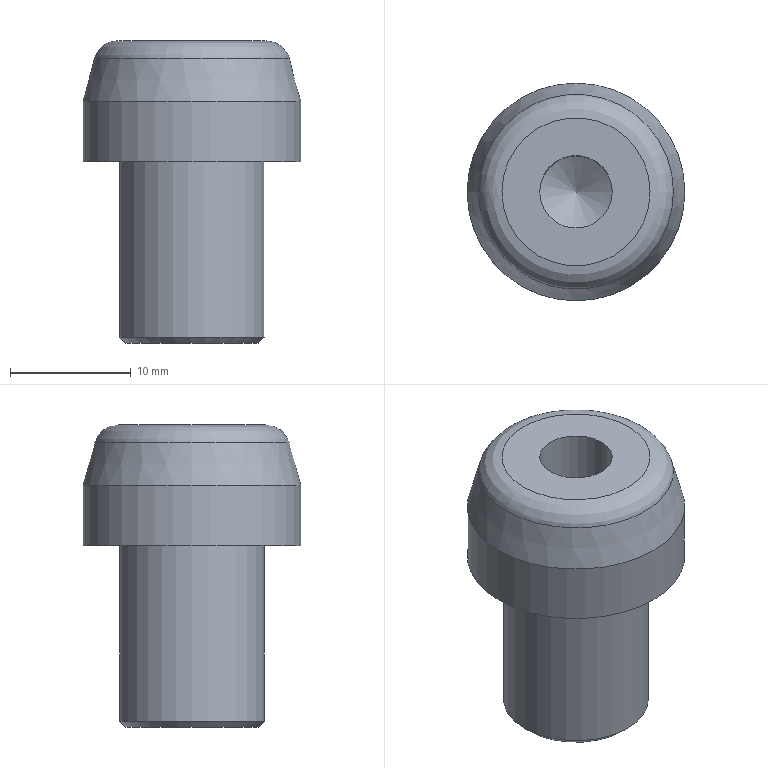Part | NX | features solid 2 | 1 solid | 10 faces | box 18 x 18 x 25 mm | volume 3736 mm3 | plane 3 | cylinder 3 | cone 3 | torus 1 | commonest cylinder face diameters 6 x1 12 x1 18 x1
STEP:
#1=CARTESIAN_POINT('',(83.131,-155.39,65.396));
#2=VERTEX_POINT('',#1);
#3=CARTESIAN_POINT('',(89.131,-155.39,65.396));
#4=DIRECTION('',(0.,0.,-1.));
#5=DIRECTION('',(-1.,0.,0.));
#6=AXIS2_PLACEMENT_3D('',#3,#4,#5);
#7=CIRCLE('',#6,6.);
#8=EDGE_CURVE('',#2,#2,#7,.T.);
#9=ORIENTED_EDGE('',*,*,#8,.F.);
#10=EDGE_LOOP('',(#9));
#11=FACE_BOUND('',#10,.T.);
#12=CARTESIAN_POINT('',(98.131,-155.39,65.396));
#13=VERTEX_POINT('',#12);
#14=CARTESIAN_POINT('',(89.131,-155.39,65.396));
#15=DIRECTION('',(0.,0.,1.));
#16=DIRECTION('',(1.,0.,0.));
#17=AXIS2_PLACEMENT_3D('',#14,#15,#16);
#18=CIRCLE('',#17,9.);
#19=EDGE_CURVE('',#13,#13,#18,.T.);
#20=ORIENTED_EDGE('',*,*,#19,.F.);
#21=EDGE_LOOP('',(#20));
#22=FACE_BOUND('',#21,.T.);
#23=CARTESIAN_POINT('',(89.131,-155.39,65.396));
#24=DIRECTION('',(0.,0.,-1.));
#25=DIRECTION('',(-1.,0.,0.));
#26=AXIS2_PLACEMENT_3D('',#23,#24,#25);
#27=PLANE('',#26);
#28=ADVANCED_FACE('',(#11,#22),#27,.T.);
#29=CARTESIAN_POINT('',(80.131,-155.39,70.396));
#30=VERTEX_POINT('',#29);
#31=CARTESIAN_POINT('',(89.131,-155.39,70.396));
#32=DIRECTION('',(0.,0.,-1.));
#33=DIRECTION('',(-1.,0.,0.));
#34=AXIS2_PLACEMENT_3D('',#31,#32,#33);
#35=CIRCLE('',#34,9.);
#36=EDGE_CURVE('',#30,#30,#35,.T.);
#37=ORIENTED_EDGE('',*,*,#36,.T.);
#38=EDGE_LOOP('',(#37));
#39=FACE_BOUND('',#38,.T.);
#40=ORIENTED_EDGE('',*,*,#19,.T.);
#41=EDGE_LOOP('',(#40));
#42=FACE_BOUND('',#41,.T.);
#43=CARTESIAN_POINT('',(89.131,-155.39,65.396));
#44=DIRECTION('',(0.,0.,1.));
#45=DIRECTION('',(1.,0.,0.));
#46=AXIS2_PLACEMENT_3D('',#43,#44,#45);
#47=CYLINDRICAL_SURFACE('',#46,9.);
#48=ADVANCED_FACE('',(#39,#42),#47,.T.);
#49=CARTESIAN_POINT('',(81.073,-155.39,73.914));
#50=VERTEX_POINT('',#49);
#51=CARTESIAN_POINT('',(89.131,-155.39,73.914));
#52=DIRECTION('',(0.,0.,-1.));
#53=DIRECTION('',(-1.,0.,0.));
#54=AXIS2_PLACEMENT_3D('',#51,#52,#53);
#55=CIRCLE('',#54,8.057);
#56=EDGE_CURVE('',#50,#50,#55,.T.);
#57=ORIENTED_EDGE('',*,*,#56,.T.);
#58=EDGE_LOOP('',(#57));
#59=FACE_BOUND('',#58,.T.);
#60=ORIENTED_EDGE('',*,*,#36,.F.);
#61=EDGE_LOOP('',(#60));
#62=FACE_BOUND('',#61,.T.);
#63=CARTESIAN_POINT('',(89.131,-155.39,70.396));
#64=DIRECTION('',(0.,0.,-1.));
#65=DIRECTION('',(1.,0.,0.));
#66=AXIS2_PLACEMENT_3D('',#63,#64,#65);
#67=CONICAL_SURFACE('',#66,9.,0.2618);
#68=ADVANCED_FACE('',(#59,#62),#67,.T.);
#69=CARTESIAN_POINT('',(86.131,-155.39,75.396));
#70=VERTEX_POINT('',#69);
#71=CARTESIAN_POINT('',(89.131,-155.39,75.396));
#72=DIRECTION('',(0.,0.,-1.));
#73=DIRECTION('',(-1.,0.,0.));
#74=AXIS2_PLACEMENT_3D('',#71,#72,#73);
#75=CIRCLE('',#74,3.);
#76=EDGE_CURVE('',#70,#70,#75,.T.);
#77=ORIENTED_EDGE('',*,*,#76,.T.);
#78=EDGE_LOOP('',(#77));
#79=FACE_BOUND('',#78,.T.);
#80=CARTESIAN_POINT('',(83.005,-155.39,75.396));
#81=VERTEX_POINT('',#80);
#82=CARTESIAN_POINT('',(89.131,-155.39,75.396));
#83=DIRECTION('',(0.,0.,-1.));
#84=DIRECTION('',(-1.,0.,0.));
#85=AXIS2_PLACEMENT_3D('',#82,#83,#84);
#86=CIRCLE('',#85,6.126);
#87=EDGE_CURVE('',#81,#81,#86,.F.);
#88=ORIENTED_EDGE('',*,*,#87,.T.);
#89=EDGE_LOOP('',(#88));
#90=FACE_BOUND('',#89,.T.);
#91=CARTESIAN_POINT('',(89.131,-155.39,75.396));
#92=DIRECTION('',(0.,0.,-1.));
#93=DIRECTION('',(-1.,0.,0.));
#94=AXIS2_PLACEMENT_3D('',#91,#92,#93);
#95=PLANE('',#94);
#96=ADVANCED_FACE('',(#79,#90),#95,.F.);
#97=CARTESIAN_POINT('',(83.631,-155.39,50.396));
#98=VERTEX_POINT('',#97);
#99=CARTESIAN_POINT('',(89.131,-155.39,50.396));
#100=DIRECTION('',(0.,0.,-1.));
#101=DIRECTION('',(-1.,0.,0.));
#102=AXIS2_PLACEMENT_3D('',#99,#100,#101);
#103=CIRCLE('',#102,5.5);
#104=EDGE_CURVE('',#98,#98,#103,.T.);
#105=ORIENTED_EDGE('',*,*,#104,.T.);
#106=EDGE_LOOP('',(#105));
#107=FACE_BOUND('',#106,.T.);
#108=CARTESIAN_POINT('',(89.131,-155.39,50.396));
#109=DIRECTION('',(0.,0.,-1.));
#110=DIRECTION('',(-1.,0.,0.));
#111=AXIS2_PLACEMENT_3D('',#108,#109,#110);
#112=PLANE('',#111);
#113=ADVANCED_FACE('',(#107),#112,.T.);
#114=CARTESIAN_POINT('',(83.131,-155.39,50.896));
#115=VERTEX_POINT('',#114);
#116=CARTESIAN_POINT('',(89.131,-155.39,50.896));
#117=DIRECTION('',(0.,0.,-1.));
#118=DIRECTION('',(-1.,0.,0.));
#119=AXIS2_PLACEMENT_3D('',#116,#117,#118);
#120=CIRCLE('',#119,6.);
#121=EDGE_CURVE('',#115,#115,#120,.F.);
#122=ORIENTED_EDGE('',*,*,#121,.T.);
#123=EDGE_LOOP('',(#122));
#124=FACE_BOUND('',#123,.T.);
#125=ORIENTED_EDGE('',*,*,#8,.T.);
#126=EDGE_LOOP('',(#125));
#127=FACE_BOUND('',#126,.T.);
#128=CARTESIAN_POINT('',(89.131,-155.39,65.396));
#129=DIRECTION('',(0.,0.,-1.));
#130=DIRECTION('',(-1.,0.,0.));
#131=AXIS2_PLACEMENT_3D('',#128,#129,#130);
#132=CYLINDRICAL_SURFACE('',#131,6.);
#133=ADVANCED_FACE('',(#124,#127),#132,.T.);
#134=ORIENTED_EDGE('',*,*,#121,.F.);
#135=EDGE_LOOP('',(#134));
#136=FACE_BOUND('',#135,.T.);
#137=ORIENTED_EDGE('',*,*,#104,.F.);
#138=EDGE_LOOP('',(#137));
#139=FACE_BOUND('',#138,.T.);
#140=CARTESIAN_POINT('',(89.131,-155.39,50.396));
#141=DIRECTION('',(0.,0.,1.));
#142=DIRECTION('',(1.,0.,0.));
#143=AXIS2_PLACEMENT_3D('',#140,#141,#142);
#144=CONICAL_SURFACE('',#143,5.5,0.7854);
#145=ADVANCED_FACE('',(#136,#139),#144,.T.);
#146=ORIENTED_EDGE('',*,*,#87,.F.);
#147=EDGE_LOOP('',(#146));
#148=FACE_BOUND('',#147,.T.);
#149=ORIENTED_EDGE('',*,*,#56,.F.);
#150=EDGE_LOOP('',(#149));
#151=FACE_BOUND('',#150,.T.);
#152=CARTESIAN_POINT('',(89.131,-155.39,73.396));
#153=DIRECTION('',(0.,0.,-1.));
#154=DIRECTION('',(-1.,0.,0.));
#155=AXIS2_PLACEMENT_3D('',#152,#153,#154);
#156=TOROIDAL_SURFACE('',#155,6.126,2.);
#157=ADVANCED_FACE('',(#148,#151),#156,.T.);
#158=CARTESIAN_POINT('',(86.131,-155.39,65.396));
#159=VERTEX_POINT('',#158);
#160=CARTESIAN_POINT('',(89.131,-155.39,65.396));
#161=DIRECTION('',(0.,0.,-1.));
#162=DIRECTION('',(-1.,0.,0.));
#163=AXIS2_PLACEMENT_3D('',#160,#161,#162);
#164=CIRCLE('',#163,3.);
#165=EDGE_CURVE('',#159,#159,#164,.T.);
#166=ORIENTED_EDGE('',*,*,#165,.F.);
#167=EDGE_LOOP('',(#166));
#168=FACE_BOUND('',#167,.T.);
#169=CARTESIAN_POINT('',(89.131,-155.39,63.593));
#170=VERTEX_POINT('',#169);
#171=VERTEX_LOOP('',#170);
#172=FACE_BOUND('',#171,.T.);
#173=CARTESIAN_POINT('',(89.131,-155.39,65.396));
#174=DIRECTION('',(0.,0.,1.));
#175=DIRECTION('',(1.,0.,0.));
#176=AXIS2_PLACEMENT_3D('',#173,#174,#175);
#177=CONICAL_SURFACE('',#176,3.,1.03);
#178=ADVANCED_FACE('',(#168,#172),#177,.F.);
#179=ORIENTED_EDGE('',*,*,#165,.T.);
#180=EDGE_LOOP('',(#179));
#181=FACE_BOUND('',#180,.T.);
#182=ORIENTED_EDGE('',*,*,#76,.F.);
#183=EDGE_LOOP('',(#182));
#184=FACE_BOUND('',#183,.T.);
#185=CARTESIAN_POINT('',(89.131,-155.39,75.396));
#186=DIRECTION('',(0.,0.,-1.));
#187=DIRECTION('',(-1.,0.,0.));
#188=AXIS2_PLACEMENT_3D('',#185,#186,#187);
#189=CYLINDRICAL_SURFACE('',#188,3.);
#190=ADVANCED_FACE('',(#181,#184),#189,.F.);
#191=CLOSED_SHELL('',(#28,#48,#68,#96,#113,#133,#145,#157,#178,#190));
#192=MANIFOLD_SOLID_BREP('',#191);
#193=(LENGTH_UNIT()NAMED_UNIT(*)SI_UNIT(.MILLI.,.METRE.));
#194=UNCERTAINTY_MEASURE_WITH_UNIT(LENGTH_MEASURE(0.00001),#193,'','');
#195=(NAMED_UNIT(*)PLANE_ANGLE_UNIT()SI_UNIT($,.RADIAN.));
#196=(NAMED_UNIT(*)SI_UNIT($,.STERADIAN.)SOLID_ANGLE_UNIT());
#197=(GEOMETRIC_REPRESENTATION_CONTEXT(3)GLOBAL_UNCERTAINTY_ASSIGNED_CONTEXT((#194))GLOBAL_UNIT_ASSIGNED_CONTEXT((#193,#195,#196))REPRESENTATION_CONTEXT('',''));
#198=ADVANCED_BREP_SHAPE_REPRESENTATION('',(#192),#197);